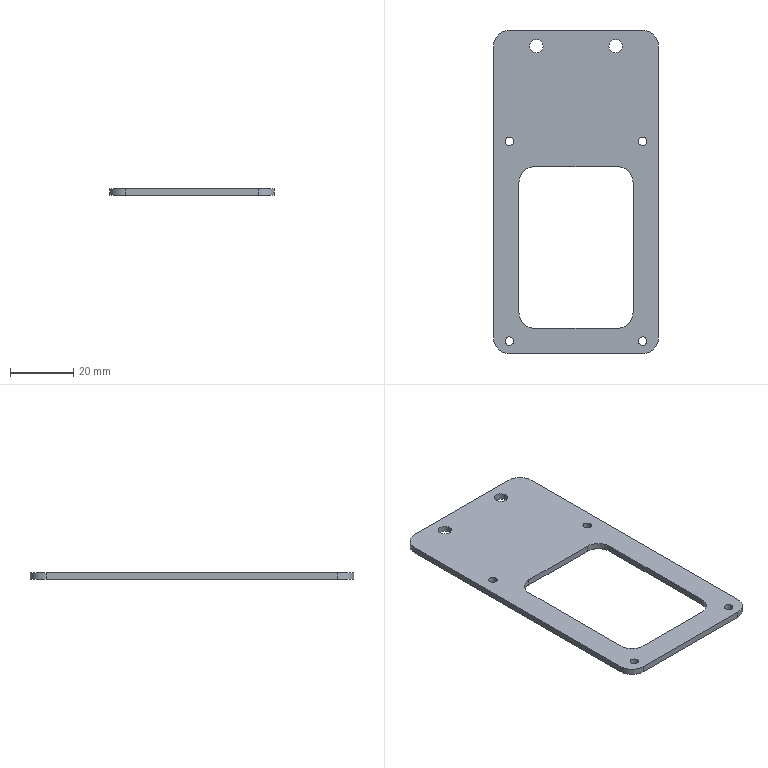Part | SolidWorks | features BaseBody 1 | 1 solid | 30 faces | box 52 x 102 x 2 mm | volume 6835 mm3 | cylinder 20 | plane 10 | commonest cylinder face diameters 2.7 x8 10 x8 4.2 x4
STEP:
#1=CARTESIAN_POINT('',(-14.6,46.,0.));
#2=VERTEX_POINT('',#1);
#3=CARTESIAN_POINT('',(-10.4,46.,0.));
#4=VERTEX_POINT('',#3);
#5=CARTESIAN_POINT('',(-12.5,46.,0.));
#6=DIRECTION('',(0.,0.,1.));
#7=DIRECTION('',(1.,0.,0.));
#8=AXIS2_PLACEMENT_3D('',#5,#6,#7);
#9=CIRCLE('',#8,2.1);
#10=EDGE_CURVE('',#2,#4,#9,.T.);
#11=ORIENTED_EDGE('',*,*,#10,.F.);
#12=CARTESIAN_POINT('',(-14.6,46.,2.));
#13=VERTEX_POINT('',#12);
#14=CARTESIAN_POINT('',(-14.6,46.,0.));
#15=DIRECTION('',(0.,0.,1.));
#16=VECTOR('',#15,1000.);
#17=LINE('',#14,#16);
#18=EDGE_CURVE('',#2,#13,#17,.T.);
#19=ORIENTED_EDGE('',*,*,#18,.T.);
#20=CARTESIAN_POINT('',(-10.4,46.,2.));
#21=VERTEX_POINT('',#20);
#22=CARTESIAN_POINT('',(-12.5,46.,2.));
#23=DIRECTION('',(0.,0.,1.));
#24=DIRECTION('',(1.,0.,0.));
#25=AXIS2_PLACEMENT_3D('',#22,#23,#24);
#26=CIRCLE('',#25,2.1);
#27=EDGE_CURVE('',#13,#21,#26,.T.);
#28=ORIENTED_EDGE('',*,*,#27,.T.);
#29=CARTESIAN_POINT('',(-10.4,46.,0.));
#30=DIRECTION('',(0.,0.,1.));
#31=VECTOR('',#30,1000.);
#32=LINE('',#29,#31);
#33=EDGE_CURVE('',#4,#21,#32,.T.);
#34=ORIENTED_EDGE('',*,*,#33,.F.);
#35=EDGE_LOOP('',(#11,#19,#28,#34));
#36=FACE_OUTER_BOUND('',#35,.T.);
#37=CARTESIAN_POINT('',(-12.5,46.,0.));
#38=DIRECTION('',(0.,0.,1.));
#39=DIRECTION('',(1.,0.,0.));
#40=AXIS2_PLACEMENT_3D('',#37,#38,#39);
#41=CYLINDRICAL_SURFACE('',#40,2.1);
#42=ADVANCED_FACE('',(#36),#41,.F.);
#43=CARTESIAN_POINT('',(19.65,-47.,0.));
#44=VERTEX_POINT('',#43);
#45=CARTESIAN_POINT('',(22.35,-47.,0.));
#46=VERTEX_POINT('',#45);
#47=CARTESIAN_POINT('',(21.,-47.,0.));
#48=DIRECTION('',(0.,0.,1.));
#49=DIRECTION('',(1.,0.,0.));
#50=AXIS2_PLACEMENT_3D('',#47,#48,#49);
#51=CIRCLE('',#50,1.35);
#52=EDGE_CURVE('',#44,#46,#51,.T.);
#53=ORIENTED_EDGE('',*,*,#52,.F.);
#54=CARTESIAN_POINT('',(19.65,-47.,2.));
#55=VERTEX_POINT('',#54);
#56=CARTESIAN_POINT('',(19.65,-47.,0.));
#57=DIRECTION('',(0.,0.,1.));
#58=VECTOR('',#57,1000.);
#59=LINE('',#56,#58);
#60=EDGE_CURVE('',#44,#55,#59,.T.);
#61=ORIENTED_EDGE('',*,*,#60,.T.);
#62=CARTESIAN_POINT('',(22.35,-47.,2.));
#63=VERTEX_POINT('',#62);
#64=CARTESIAN_POINT('',(21.,-47.,2.));
#65=DIRECTION('',(0.,0.,1.));
#66=DIRECTION('',(1.,0.,0.));
#67=AXIS2_PLACEMENT_3D('',#64,#65,#66);
#68=CIRCLE('',#67,1.35);
#69=EDGE_CURVE('',#55,#63,#68,.T.);
#70=ORIENTED_EDGE('',*,*,#69,.T.);
#71=CARTESIAN_POINT('',(22.35,-47.,0.));
#72=DIRECTION('',(0.,0.,1.));
#73=VECTOR('',#72,1000.);
#74=LINE('',#71,#73);
#75=EDGE_CURVE('',#46,#63,#74,.T.);
#76=ORIENTED_EDGE('',*,*,#75,.F.);
#77=EDGE_LOOP('',(#53,#61,#70,#76));
#78=FACE_OUTER_BOUND('',#77,.T.);
#79=CARTESIAN_POINT('',(21.,-47.,0.));
#80=DIRECTION('',(0.,0.,1.));
#81=DIRECTION('',(1.,0.,0.));
#82=AXIS2_PLACEMENT_3D('',#79,#80,#81);
#83=CYLINDRICAL_SURFACE('',#82,1.35);
#84=ADVANCED_FACE('',(#78),#83,.F.);
#85=CARTESIAN_POINT('',(10.4,46.,0.));
#86=VERTEX_POINT('',#85);
#87=CARTESIAN_POINT('',(14.6,46.,0.));
#88=VERTEX_POINT('',#87);
#89=CARTESIAN_POINT('',(12.5,46.,0.));
#90=DIRECTION('',(0.,0.,1.));
#91=DIRECTION('',(1.,0.,0.));
#92=AXIS2_PLACEMENT_3D('',#89,#90,#91);
#93=CIRCLE('',#92,2.1);
#94=EDGE_CURVE('',#86,#88,#93,.T.);
#95=ORIENTED_EDGE('',*,*,#94,.F.);
#96=CARTESIAN_POINT('',(10.4,46.,2.));
#97=VERTEX_POINT('',#96);
#98=CARTESIAN_POINT('',(10.4,46.,0.));
#99=DIRECTION('',(0.,0.,1.));
#100=VECTOR('',#99,1000.);
#101=LINE('',#98,#100);
#102=EDGE_CURVE('',#86,#97,#101,.T.);
#103=ORIENTED_EDGE('',*,*,#102,.T.);
#104=CARTESIAN_POINT('',(14.6,46.,2.));
#105=VERTEX_POINT('',#104);
#106=CARTESIAN_POINT('',(12.5,46.,2.));
#107=DIRECTION('',(0.,0.,1.));
#108=DIRECTION('',(1.,0.,0.));
#109=AXIS2_PLACEMENT_3D('',#106,#107,#108);
#110=CIRCLE('',#109,2.1);
#111=EDGE_CURVE('',#97,#105,#110,.T.);
#112=ORIENTED_EDGE('',*,*,#111,.T.);
#113=CARTESIAN_POINT('',(14.6,46.,0.));
#114=DIRECTION('',(0.,0.,1.));
#115=VECTOR('',#114,1000.);
#116=LINE('',#113,#115);
#117=EDGE_CURVE('',#88,#105,#116,.T.);
#118=ORIENTED_EDGE('',*,*,#117,.F.);
#119=EDGE_LOOP('',(#95,#103,#112,#118));
#120=FACE_OUTER_BOUND('',#119,.T.);
#121=CARTESIAN_POINT('',(12.5,46.,0.));
#122=DIRECTION('',(0.,0.,1.));
#123=DIRECTION('',(1.,0.,0.));
#124=AXIS2_PLACEMENT_3D('',#121,#122,#123);
#125=CYLINDRICAL_SURFACE('',#124,2.1);
#126=ADVANCED_FACE('',(#120),#125,.F.);
#127=CARTESIAN_POINT('',(-22.35,16.,0.));
#128=VERTEX_POINT('',#127);
#129=CARTESIAN_POINT('',(-19.65,16.,0.));
#130=VERTEX_POINT('',#129);
#131=CARTESIAN_POINT('',(-21.,16.,0.));
#132=DIRECTION('',(0.,0.,1.));
#133=DIRECTION('',(1.,0.,0.));
#134=AXIS2_PLACEMENT_3D('',#131,#132,#133);
#135=CIRCLE('',#134,1.35);
#136=EDGE_CURVE('',#128,#130,#135,.T.);
#137=ORIENTED_EDGE('',*,*,#136,.F.);
#138=CARTESIAN_POINT('',(-22.35,16.,2.));
#139=VERTEX_POINT('',#138);
#140=CARTESIAN_POINT('',(-22.35,16.,0.));
#141=DIRECTION('',(0.,0.,1.));
#142=VECTOR('',#141,1000.);
#143=LINE('',#140,#142);
#144=EDGE_CURVE('',#128,#139,#143,.T.);
#145=ORIENTED_EDGE('',*,*,#144,.T.);
#146=CARTESIAN_POINT('',(-19.65,16.,2.));
#147=VERTEX_POINT('',#146);
#148=CARTESIAN_POINT('',(-21.,16.,2.));
#149=DIRECTION('',(0.,0.,1.));
#150=DIRECTION('',(1.,0.,0.));
#151=AXIS2_PLACEMENT_3D('',#148,#149,#150);
#152=CIRCLE('',#151,1.35);
#153=EDGE_CURVE('',#139,#147,#152,.T.);
#154=ORIENTED_EDGE('',*,*,#153,.T.);
#155=CARTESIAN_POINT('',(-19.65,16.,0.));
#156=DIRECTION('',(0.,0.,1.));
#157=VECTOR('',#156,1000.);
#158=LINE('',#155,#157);
#159=EDGE_CURVE('',#130,#147,#158,.T.);
#160=ORIENTED_EDGE('',*,*,#159,.F.);
#161=EDGE_LOOP('',(#137,#145,#154,#160));
#162=FACE_OUTER_BOUND('',#161,.T.);
#163=CARTESIAN_POINT('',(-21.,16.,0.));
#164=DIRECTION('',(0.,0.,1.));
#165=DIRECTION('',(1.,0.,0.));
#166=AXIS2_PLACEMENT_3D('',#163,#164,#165);
#167=CYLINDRICAL_SURFACE('',#166,1.35);
#168=ADVANCED_FACE('',(#162),#167,.F.);
#169=CARTESIAN_POINT('',(19.65,16.,0.));
#170=VERTEX_POINT('',#169);
#171=CARTESIAN_POINT('',(22.35,16.,0.));
#172=VERTEX_POINT('',#171);
#173=CARTESIAN_POINT('',(21.,16.,0.));
#174=DIRECTION('',(0.,0.,1.));
#175=DIRECTION('',(1.,0.,0.));
#176=AXIS2_PLACEMENT_3D('',#173,#174,#175);
#177=CIRCLE('',#176,1.35);
#178=EDGE_CURVE('',#170,#172,#177,.T.);
#179=ORIENTED_EDGE('',*,*,#178,.F.);
#180=CARTESIAN_POINT('',(19.65,16.,2.));
#181=VERTEX_POINT('',#180);
#182=CARTESIAN_POINT('',(19.65,16.,0.));
#183=DIRECTION('',(0.,0.,1.));
#184=VECTOR('',#183,1000.);
#185=LINE('',#182,#184);
#186=EDGE_CURVE('',#170,#181,#185,.T.);
#187=ORIENTED_EDGE('',*,*,#186,.T.);
#188=CARTESIAN_POINT('',(22.35,16.,2.));
#189=VERTEX_POINT('',#188);
#190=CARTESIAN_POINT('',(21.,16.,2.));
#191=DIRECTION('',(0.,0.,1.));
#192=DIRECTION('',(1.,0.,0.));
#193=AXIS2_PLACEMENT_3D('',#190,#191,#192);
#194=CIRCLE('',#193,1.35);
#195=EDGE_CURVE('',#181,#189,#194,.T.);
#196=ORIENTED_EDGE('',*,*,#195,.T.);
#197=CARTESIAN_POINT('',(22.35,16.,0.));
#198=DIRECTION('',(0.,0.,1.));
#199=VECTOR('',#198,1000.);
#200=LINE('',#197,#199);
#201=EDGE_CURVE('',#172,#189,#200,.T.);
#202=ORIENTED_EDGE('',*,*,#201,.F.);
#203=EDGE_LOOP('',(#179,#187,#196,#202));
#204=FACE_OUTER_BOUND('',#203,.T.);
#205=CARTESIAN_POINT('',(21.,16.,0.));
#206=DIRECTION('',(0.,0.,1.));
#207=DIRECTION('',(1.,0.,0.));
#208=AXIS2_PLACEMENT_3D('',#205,#206,#207);
#209=CYLINDRICAL_SURFACE('',#208,1.35);
#210=ADVANCED_FACE('',(#204),#209,.F.);
#211=CARTESIAN_POINT('',(-22.35,-47.,0.));
#212=VERTEX_POINT('',#211);
#213=CARTESIAN_POINT('',(-19.65,-47.,0.));
#214=VERTEX_POINT('',#213);
#215=CARTESIAN_POINT('',(-21.,-47.,0.));
#216=DIRECTION('',(0.,0.,1.));
#217=DIRECTION('',(1.,0.,0.));
#218=AXIS2_PLACEMENT_3D('',#215,#216,#217);
#219=CIRCLE('',#218,1.35);
#220=EDGE_CURVE('',#212,#214,#219,.T.);
#221=ORIENTED_EDGE('',*,*,#220,.F.);
#222=CARTESIAN_POINT('',(-22.35,-47.,2.));
#223=VERTEX_POINT('',#222);
#224=CARTESIAN_POINT('',(-22.35,-47.,0.));
#225=DIRECTION('',(0.,0.,1.));
#226=VECTOR('',#225,1000.);
#227=LINE('',#224,#226);
#228=EDGE_CURVE('',#212,#223,#227,.T.);
#229=ORIENTED_EDGE('',*,*,#228,.T.);
#230=CARTESIAN_POINT('',(-19.65,-47.,2.));
#231=VERTEX_POINT('',#230);
#232=CARTESIAN_POINT('',(-21.,-47.,2.));
#233=DIRECTION('',(0.,0.,1.));
#234=DIRECTION('',(1.,0.,0.));
#235=AXIS2_PLACEMENT_3D('',#232,#233,#234);
#236=CIRCLE('',#235,1.35);
#237=EDGE_CURVE('',#223,#231,#236,.T.);
#238=ORIENTED_EDGE('',*,*,#237,.T.);
#239=CARTESIAN_POINT('',(-19.65,-47.,0.));
#240=DIRECTION('',(0.,0.,1.));
#241=VECTOR('',#240,1000.);
#242=LINE('',#239,#241);
#243=EDGE_CURVE('',#214,#231,#242,.T.);
#244=ORIENTED_EDGE('',*,*,#243,.F.);
#245=EDGE_LOOP('',(#221,#229,#238,#244));
#246=FACE_OUTER_BOUND('',#245,.T.);
#247=CARTESIAN_POINT('',(-21.,-47.,0.));
#248=DIRECTION('',(0.,0.,1.));
#249=DIRECTION('',(1.,0.,0.));
#250=AXIS2_PLACEMENT_3D('',#247,#248,#249);
#251=CYLINDRICAL_SURFACE('',#250,1.35);
#252=ADVANCED_FACE('',(#246),#251,.F.);
#253=CARTESIAN_POINT('',(-21.,-51.,2.));
#254=VERTEX_POINT('',#253);
#255=CARTESIAN_POINT('',(-26.,-46.,2.));
#256=VERTEX_POINT('',#255);
#257=CARTESIAN_POINT('',(-21.,-46.,2.));
#258=DIRECTION('',(0.,0.,-1.));
#259=DIRECTION('',(-1.,0.,0.));
#260=AXIS2_PLACEMENT_3D('',#257,#258,#259);
#261=CIRCLE('',#260,5.);
#262=EDGE_CURVE('',#254,#256,#261,.T.);
#263=ORIENTED_EDGE('',*,*,#262,.F.);
#264=CARTESIAN_POINT('',(21.,-51.,2.));
#265=VERTEX_POINT('',#264);
#266=CARTESIAN_POINT('',(0.,-51.,2.));
#267=DIRECTION('',(-1.,0.,0.));
#268=VECTOR('',#267,1000.);
#269=LINE('',#266,#268);
#270=EDGE_CURVE('',#265,#254,#269,.T.);
#271=ORIENTED_EDGE('',*,*,#270,.F.);
#272=CARTESIAN_POINT('',(26.,-46.,2.));
#273=VERTEX_POINT('',#272);
#274=CARTESIAN_POINT('',(21.,-46.,2.));
#275=DIRECTION('',(0.,0.,-1.));
#276=DIRECTION('',(-1.,0.,0.));
#277=AXIS2_PLACEMENT_3D('',#274,#275,#276);
#278=CIRCLE('',#277,5.);
#279=EDGE_CURVE('',#273,#265,#278,.T.);
#280=ORIENTED_EDGE('',*,*,#279,.F.);
#281=CARTESIAN_POINT('',(26.,46.,2.));
#282=VERTEX_POINT('',#281);
#283=CARTESIAN_POINT('',(26.,0.,2.));
#284=DIRECTION('',(0.,-1.,0.));
#285=VECTOR('',#284,1000.);
#286=LINE('',#283,#285);
#287=EDGE_CURVE('',#282,#273,#286,.T.);
#288=ORIENTED_EDGE('',*,*,#287,.F.);
#289=CARTESIAN_POINT('',(21.,51.,2.));
#290=VERTEX_POINT('',#289);
#291=CARTESIAN_POINT('',(21.,46.,2.));
#292=DIRECTION('',(0.,0.,-1.));
#293=DIRECTION('',(-1.,0.,0.));
#294=AXIS2_PLACEMENT_3D('',#291,#292,#293);
#295=CIRCLE('',#294,5.);
#296=EDGE_CURVE('',#290,#282,#295,.T.);
#297=ORIENTED_EDGE('',*,*,#296,.F.);
#298=CARTESIAN_POINT('',(-21.,51.,2.));
#299=VERTEX_POINT('',#298);
#300=CARTESIAN_POINT('',(0.,51.,2.));
#301=DIRECTION('',(1.,0.,0.));
#302=VECTOR('',#301,1000.);
#303=LINE('',#300,#302);
#304=EDGE_CURVE('',#299,#290,#303,.T.);
#305=ORIENTED_EDGE('',*,*,#304,.F.);
#306=CARTESIAN_POINT('',(-26.,46.,2.));
#307=VERTEX_POINT('',#306);
#308=CARTESIAN_POINT('',(-21.,46.,2.));
#309=DIRECTION('',(0.,0.,-1.));
#310=DIRECTION('',(-1.,0.,0.));
#311=AXIS2_PLACEMENT_3D('',#308,#309,#310);
#312=CIRCLE('',#311,5.);
#313=EDGE_CURVE('',#307,#299,#312,.T.);
#314=ORIENTED_EDGE('',*,*,#313,.F.);
#315=CARTESIAN_POINT('',(-26.,0.,2.));
#316=DIRECTION('',(0.,1.,0.));
#317=VECTOR('',#316,1000.);
#318=LINE('',#315,#317);
#319=EDGE_CURVE('',#256,#307,#318,.T.);
#320=ORIENTED_EDGE('',*,*,#319,.F.);
#321=EDGE_LOOP('',(#263,#271,#280,#288,#297,#305,#314,#320));
#322=FACE_OUTER_BOUND('',#321,.T.);
#323=CARTESIAN_POINT('',(-12.5,46.,2.));
#324=DIRECTION('',(0.,0.,1.));
#325=DIRECTION('',(1.,0.,0.));
#326=AXIS2_PLACEMENT_3D('',#323,#324,#325);
#327=CIRCLE('',#326,2.1);
#328=EDGE_CURVE('',#21,#13,#327,.T.);
#329=ORIENTED_EDGE('',*,*,#328,.F.);
#330=ORIENTED_EDGE('',*,*,#27,.F.);
#331=EDGE_LOOP('',(#329,#330));
#332=FACE_BOUND('',#331,.T.);
#333=CARTESIAN_POINT('',(21.,-47.,2.));
#334=DIRECTION('',(0.,0.,1.));
#335=DIRECTION('',(1.,0.,0.));
#336=AXIS2_PLACEMENT_3D('',#333,#334,#335);
#337=CIRCLE('',#336,1.35);
#338=EDGE_CURVE('',#63,#55,#337,.T.);
#339=ORIENTED_EDGE('',*,*,#338,.F.);
#340=ORIENTED_EDGE('',*,*,#69,.F.);
#341=EDGE_LOOP('',(#339,#340));
#342=FACE_BOUND('',#341,.T.);
#343=CARTESIAN_POINT('',(12.5,46.,2.));
#344=DIRECTION('',(0.,0.,1.));
#345=DIRECTION('',(1.,0.,0.));
#346=AXIS2_PLACEMENT_3D('',#343,#344,#345);
#347=CIRCLE('',#346,2.1);
#348=EDGE_CURVE('',#105,#97,#347,.T.);
#349=ORIENTED_EDGE('',*,*,#348,.F.);
#350=ORIENTED_EDGE('',*,*,#111,.F.);
#351=EDGE_LOOP('',(#349,#350));
#352=FACE_BOUND('',#351,.T.);
#353=CARTESIAN_POINT('',(-21.,16.,2.));
#354=DIRECTION('',(0.,0.,1.));
#355=DIRECTION('',(1.,0.,0.));
#356=AXIS2_PLACEMENT_3D('',#353,#354,#355);
#357=CIRCLE('',#356,1.35);
#358=EDGE_CURVE('',#147,#139,#357,.T.);
#359=ORIENTED_EDGE('',*,*,#358,.F.);
#360=ORIENTED_EDGE('',*,*,#153,.F.);
#361=EDGE_LOOP('',(#359,#360));
#362=FACE_BOUND('',#361,.T.);
#363=CARTESIAN_POINT('',(21.,16.,2.));
#364=DIRECTION('',(0.,0.,1.));
#365=DIRECTION('',(1.,0.,0.));
#366=AXIS2_PLACEMENT_3D('',#363,#364,#365);
#367=CIRCLE('',#366,1.35);
#368=EDGE_CURVE('',#189,#181,#367,.T.);
#369=ORIENTED_EDGE('',*,*,#368,.F.);
#370=ORIENTED_EDGE('',*,*,#195,.F.);
#371=EDGE_LOOP('',(#369,#370));
#372=FACE_BOUND('',#371,.T.);
#373=CARTESIAN_POINT('',(-21.,-47.,2.));
#374=DIRECTION('',(0.,0.,1.));
#375=DIRECTION('',(1.,0.,0.));
#376=AXIS2_PLACEMENT_3D('',#373,#374,#375);
#377=CIRCLE('',#376,1.35);
#378=EDGE_CURVE('',#231,#223,#377,.T.);
#379=ORIENTED_EDGE('',*,*,#378,.F.);
#380=ORIENTED_EDGE('',*,*,#237,.F.);
#381=EDGE_LOOP('',(#379,#380));
#382=FACE_BOUND('',#381,.T.);
#383=CARTESIAN_POINT('',(18.,3.,2.));
#384=VERTEX_POINT('',#383);
#385=CARTESIAN_POINT('',(13.,8.,2.));
#386=VERTEX_POINT('',#385);
#387=CARTESIAN_POINT('',(13.,3.,2.));
#388=DIRECTION('',(0.,0.,1.));
#389=DIRECTION('',(-1.,0.,0.));
#390=AXIS2_PLACEMENT_3D('',#387,#388,#389);
#391=CIRCLE('',#390,5.);
#392=EDGE_CURVE('',#384,#386,#391,.T.);
#393=ORIENTED_EDGE('',*,*,#392,.F.);
#394=CARTESIAN_POINT('',(18.,-38.,2.));
#395=VERTEX_POINT('',#394);
#396=CARTESIAN_POINT('',(18.,0.,2.));
#397=DIRECTION('',(0.,1.,0.));
#398=VECTOR('',#397,1000.);
#399=LINE('',#396,#398);
#400=EDGE_CURVE('',#395,#384,#399,.T.);
#401=ORIENTED_EDGE('',*,*,#400,.F.);
#402=CARTESIAN_POINT('',(13.,-43.,2.));
#403=VERTEX_POINT('',#402);
#404=CARTESIAN_POINT('',(13.,-38.,2.));
#405=DIRECTION('',(0.,0.,1.));
#406=DIRECTION('',(-1.,0.,0.));
#407=AXIS2_PLACEMENT_3D('',#404,#405,#406);
#408=CIRCLE('',#407,5.);
#409=EDGE_CURVE('',#403,#395,#408,.T.);
#410=ORIENTED_EDGE('',*,*,#409,.F.);
#411=CARTESIAN_POINT('',(-13.,-43.,2.));
#412=VERTEX_POINT('',#411);
#413=CARTESIAN_POINT('',(0.,-43.,2.));
#414=DIRECTION('',(1.,0.,0.));
#415=VECTOR('',#414,1000.);
#416=LINE('',#413,#415);
#417=EDGE_CURVE('',#412,#403,#416,.T.);
#418=ORIENTED_EDGE('',*,*,#417,.F.);
#419=CARTESIAN_POINT('',(-18.,-38.,2.));
#420=VERTEX_POINT('',#419);
#421=CARTESIAN_POINT('',(-13.,-38.,2.));
#422=DIRECTION('',(0.,0.,1.));
#423=DIRECTION('',(-1.,0.,0.));
#424=AXIS2_PLACEMENT_3D('',#421,#422,#423);
#425=CIRCLE('',#424,5.);
#426=EDGE_CURVE('',#420,#412,#425,.T.);
#427=ORIENTED_EDGE('',*,*,#426,.F.);
#428=CARTESIAN_POINT('',(-18.,3.,2.));
#429=VERTEX_POINT('',#428);
#430=CARTESIAN_POINT('',(-18.,0.,2.));
#431=DIRECTION('',(0.,-1.,0.));
#432=VECTOR('',#431,1000.);
#433=LINE('',#430,#432);
#434=EDGE_CURVE('',#429,#420,#433,.T.);
#435=ORIENTED_EDGE('',*,*,#434,.F.);
#436=CARTESIAN_POINT('',(-13.,8.,2.));
#437=VERTEX_POINT('',#436);
#438=CARTESIAN_POINT('',(-13.,3.,2.));
#439=DIRECTION('',(0.,0.,1.));
#440=DIRECTION('',(-1.,0.,0.));
#441=AXIS2_PLACEMENT_3D('',#438,#439,#440);
#442=CIRCLE('',#441,5.);
#443=EDGE_CURVE('',#437,#429,#442,.T.);
#444=ORIENTED_EDGE('',*,*,#443,.F.);
#445=CARTESIAN_POINT('',(0.,8.,2.));
#446=DIRECTION('',(-1.,0.,0.));
#447=VECTOR('',#446,1000.);
#448=LINE('',#445,#447);
#449=EDGE_CURVE('',#386,#437,#448,.T.);
#450=ORIENTED_EDGE('',*,*,#449,.F.);
#451=EDGE_LOOP('',(#393,#401,#410,#418,#427,#435,#444,#450));
#452=FACE_BOUND('',#451,.T.);
#453=CARTESIAN_POINT('',(0.,0.,2.));
#454=DIRECTION('',(0.,0.,-1.));
#455=DIRECTION('',(-1.,0.,0.));
#456=AXIS2_PLACEMENT_3D('',#453,#454,#455);
#457=PLANE('',#456);
#458=ADVANCED_FACE('',(#322,#332,#342,#352,#362,#372,#382,#452),#457,.F.);
#459=CARTESIAN_POINT('',(-26.,-46.,0.));
#460=VERTEX_POINT('',#459);
#461=CARTESIAN_POINT('',(-26.,-46.,2.));
#462=DIRECTION('',(0.,0.,-1.));
#463=VECTOR('',#462,1000.);
#464=LINE('',#461,#463);
#465=EDGE_CURVE('',#256,#460,#464,.T.);
#466=ORIENTED_EDGE('',*,*,#465,.F.);
#467=ORIENTED_EDGE('',*,*,#319,.T.);
#468=CARTESIAN_POINT('',(-26.,46.,0.));
#469=VERTEX_POINT('',#468);
#470=CARTESIAN_POINT('',(-26.,46.,2.));
#471=DIRECTION('',(0.,0.,1.));
#472=VECTOR('',#471,1000.);
#473=LINE('',#470,#472);
#474=EDGE_CURVE('',#469,#307,#473,.T.);
#475=ORIENTED_EDGE('',*,*,#474,.F.);
#476=CARTESIAN_POINT('',(-26.,-51.,0.));
#477=DIRECTION('',(0.,1.,0.));
#478=VECTOR('',#477,1000.);
#479=LINE('',#476,#478);
#480=EDGE_CURVE('',#460,#469,#479,.T.);
#481=ORIENTED_EDGE('',*,*,#480,.F.);
#482=EDGE_LOOP('',(#466,#467,#475,#481));
#483=FACE_OUTER_BOUND('',#482,.T.);
#484=CARTESIAN_POINT('',(-26.,-51.,2.));
#485=DIRECTION('',(1.,0.,0.));
#486=DIRECTION('',(0.,0.,-1.));
#487=AXIS2_PLACEMENT_3D('',#484,#485,#486);
#488=PLANE('',#487);
#489=ADVANCED_FACE('',(#483),#488,.F.);
#490=CARTESIAN_POINT('',(-21.,-51.,0.));
#491=VERTEX_POINT('',#490);
#492=CARTESIAN_POINT('',(-21.,-46.,0.));
#493=DIRECTION('',(0.,0.,1.));
#494=DIRECTION('',(-1.,0.,0.));
#495=AXIS2_PLACEMENT_3D('',#492,#493,#494);
#496=CIRCLE('',#495,5.);
#497=EDGE_CURVE('',#460,#491,#496,.T.);
#498=ORIENTED_EDGE('',*,*,#497,.T.);
#499=CARTESIAN_POINT('',(-21.,-51.,2.));
#500=DIRECTION('',(0.,0.,1.));
#501=VECTOR('',#500,1000.);
#502=LINE('',#499,#501);
#503=EDGE_CURVE('',#491,#254,#502,.T.);
#504=ORIENTED_EDGE('',*,*,#503,.T.);
#505=ORIENTED_EDGE('',*,*,#262,.T.);
#506=ORIENTED_EDGE('',*,*,#465,.T.);
#507=EDGE_LOOP('',(#498,#504,#505,#506));
#508=FACE_OUTER_BOUND('',#507,.T.);
#509=CARTESIAN_POINT('',(-21.,-46.,2.));
#510=DIRECTION('',(0.,0.,-1.));
#511=DIRECTION('',(-1.,0.,0.));
#512=AXIS2_PLACEMENT_3D('',#509,#510,#511);
#513=CYLINDRICAL_SURFACE('',#512,5.);
#514=ADVANCED_FACE('',(#508),#513,.T.);
#515=ORIENTED_EDGE('',*,*,#503,.F.);
#516=CARTESIAN_POINT('',(21.,-51.,0.));
#517=VERTEX_POINT('',#516);
#518=CARTESIAN_POINT('',(-26.,-51.,0.));
#519=DIRECTION('',(-1.,0.,0.));
#520=VECTOR('',#519,1000.);
#521=LINE('',#518,#520);
#522=EDGE_CURVE('',#517,#491,#521,.T.);
#523=ORIENTED_EDGE('',*,*,#522,.F.);
#524=CARTESIAN_POINT('',(21.,-51.,2.));
#525=DIRECTION('',(0.,0.,-1.));
#526=VECTOR('',#525,1000.);
#527=LINE('',#524,#526);
#528=EDGE_CURVE('',#265,#517,#527,.T.);
#529=ORIENTED_EDGE('',*,*,#528,.F.);
#530=ORIENTED_EDGE('',*,*,#270,.T.);
#531=EDGE_LOOP('',(#515,#523,#529,#530));
#532=FACE_OUTER_BOUND('',#531,.T.);
#533=CARTESIAN_POINT('',(-26.,-51.,2.));
#534=DIRECTION('',(0.,1.,0.));
#535=DIRECTION('',(0.,0.,1.));
#536=AXIS2_PLACEMENT_3D('',#533,#534,#535);
#537=PLANE('',#536);
#538=ADVANCED_FACE('',(#532),#537,.F.);
#539=CARTESIAN_POINT('',(26.,-46.,0.));
#540=VERTEX_POINT('',#539);
#541=CARTESIAN_POINT('',(21.,-46.,0.));
#542=DIRECTION('',(0.,0.,1.));
#543=DIRECTION('',(-1.,0.,0.));
#544=AXIS2_PLACEMENT_3D('',#541,#542,#543);
#545=CIRCLE('',#544,5.);
#546=EDGE_CURVE('',#517,#540,#545,.T.);
#547=ORIENTED_EDGE('',*,*,#546,.T.);
#548=CARTESIAN_POINT('',(26.,-46.,2.));
#549=DIRECTION('',(0.,0.,1.));
#550=VECTOR('',#549,1000.);
#551=LINE('',#548,#550);
#552=EDGE_CURVE('',#540,#273,#551,.T.);
#553=ORIENTED_EDGE('',*,*,#552,.T.);
#554=ORIENTED_EDGE('',*,*,#279,.T.);
#555=ORIENTED_EDGE('',*,*,#528,.T.);
#556=EDGE_LOOP('',(#547,#553,#554,#555));
#557=FACE_OUTER_BOUND('',#556,.T.);
#558=CARTESIAN_POINT('',(21.,-46.,2.));
#559=DIRECTION('',(0.,0.,-1.));
#560=DIRECTION('',(-1.,0.,0.));
#561=AXIS2_PLACEMENT_3D('',#558,#559,#560);
#562=CYLINDRICAL_SURFACE('',#561,5.);
#563=ADVANCED_FACE('',(#557),#562,.T.);
#564=ORIENTED_EDGE('',*,*,#552,.F.);
#565=CARTESIAN_POINT('',(26.,46.,0.));
#566=VERTEX_POINT('',#565);
#567=CARTESIAN_POINT('',(26.,-51.,0.));
#568=DIRECTION('',(0.,-1.,0.));
#569=VECTOR('',#568,1000.);
#570=LINE('',#567,#569);
#571=EDGE_CURVE('',#566,#540,#570,.T.);
#572=ORIENTED_EDGE('',*,*,#571,.F.);
#573=CARTESIAN_POINT('',(26.,46.,2.));
#574=DIRECTION('',(0.,0.,-1.));
#575=VECTOR('',#574,1000.);
#576=LINE('',#573,#575);
#577=EDGE_CURVE('',#282,#566,#576,.T.);
#578=ORIENTED_EDGE('',*,*,#577,.F.);
#579=ORIENTED_EDGE('',*,*,#287,.T.);
#580=EDGE_LOOP('',(#564,#572,#578,#579));
#581=FACE_OUTER_BOUND('',#580,.T.);
#582=CARTESIAN_POINT('',(26.,-51.,2.));
#583=DIRECTION('',(-1.,0.,0.));
#584=DIRECTION('',(0.,0.,1.));
#585=AXIS2_PLACEMENT_3D('',#582,#583,#584);
#586=PLANE('',#585);
#587=ADVANCED_FACE('',(#581),#586,.F.);
#588=CARTESIAN_POINT('',(21.,51.,0.));
#589=VERTEX_POINT('',#588);
#590=CARTESIAN_POINT('',(21.,46.,0.));
#591=DIRECTION('',(0.,0.,1.));
#592=DIRECTION('',(-1.,0.,0.));
#593=AXIS2_PLACEMENT_3D('',#590,#591,#592);
#594=CIRCLE('',#593,5.);
#595=EDGE_CURVE('',#566,#589,#594,.T.);
#596=ORIENTED_EDGE('',*,*,#595,.T.);
#597=CARTESIAN_POINT('',(21.,51.,2.));
#598=DIRECTION('',(0.,0.,1.));
#599=VECTOR('',#598,1000.);
#600=LINE('',#597,#599);
#601=EDGE_CURVE('',#589,#290,#600,.T.);
#602=ORIENTED_EDGE('',*,*,#601,.T.);
#603=ORIENTED_EDGE('',*,*,#296,.T.);
#604=ORIENTED_EDGE('',*,*,#577,.T.);
#605=EDGE_LOOP('',(#596,#602,#603,#604));
#606=FACE_OUTER_BOUND('',#605,.T.);
#607=CARTESIAN_POINT('',(21.,46.,2.));
#608=DIRECTION('',(0.,0.,-1.));
#609=DIRECTION('',(-1.,0.,0.));
#610=AXIS2_PLACEMENT_3D('',#607,#608,#609);
#611=CYLINDRICAL_SURFACE('',#610,5.);
#612=ADVANCED_FACE('',(#606),#611,.T.);
#613=CARTESIAN_POINT('',(-21.,51.,0.));
#614=VERTEX_POINT('',#613);
#615=CARTESIAN_POINT('',(-21.,51.,2.));
#616=DIRECTION('',(0.,0.,-1.));
#617=VECTOR('',#616,1000.);
#618=LINE('',#615,#617);
#619=EDGE_CURVE('',#299,#614,#618,.T.);
#620=ORIENTED_EDGE('',*,*,#619,.F.);
#621=ORIENTED_EDGE('',*,*,#304,.T.);
#622=ORIENTED_EDGE('',*,*,#601,.F.);
#623=CARTESIAN_POINT('',(-26.,51.,0.));
#624=DIRECTION('',(1.,0.,0.));
#625=VECTOR('',#624,1000.);
#626=LINE('',#623,#625);
#627=EDGE_CURVE('',#614,#589,#626,.T.);
#628=ORIENTED_EDGE('',*,*,#627,.F.);
#629=EDGE_LOOP('',(#620,#621,#622,#628));
#630=FACE_OUTER_BOUND('',#629,.T.);
#631=CARTESIAN_POINT('',(-26.,51.,2.));
#632=DIRECTION('',(0.,-1.,0.));
#633=DIRECTION('',(0.,0.,-1.));
#634=AXIS2_PLACEMENT_3D('',#631,#632,#633);
#635=PLANE('',#634);
#636=ADVANCED_FACE('',(#630),#635,.F.);
#637=CARTESIAN_POINT('',(-21.,46.,0.));
#638=DIRECTION('',(0.,0.,1.));
#639=DIRECTION('',(-1.,0.,0.));
#640=AXIS2_PLACEMENT_3D('',#637,#638,#639);
#641=CIRCLE('',#640,5.);
#642=EDGE_CURVE('',#614,#469,#641,.T.);
#643=ORIENTED_EDGE('',*,*,#642,.T.);
#644=ORIENTED_EDGE('',*,*,#474,.T.);
#645=ORIENTED_EDGE('',*,*,#313,.T.);
#646=ORIENTED_EDGE('',*,*,#619,.T.);
#647=EDGE_LOOP('',(#643,#644,#645,#646));
#648=FACE_OUTER_BOUND('',#647,.T.);
#649=CARTESIAN_POINT('',(-21.,46.,2.));
#650=DIRECTION('',(0.,0.,-1.));
#651=DIRECTION('',(-1.,0.,0.));
#652=AXIS2_PLACEMENT_3D('',#649,#650,#651);
#653=CYLINDRICAL_SURFACE('',#652,5.);
#654=ADVANCED_FACE('',(#648),#653,.T.);
#655=ORIENTED_EDGE('',*,*,#18,.F.);
#656=CARTESIAN_POINT('',(-12.5,46.,0.));
#657=DIRECTION('',(0.,0.,1.));
#658=DIRECTION('',(1.,0.,0.));
#659=AXIS2_PLACEMENT_3D('',#656,#657,#658);
#660=CIRCLE('',#659,2.1);
#661=EDGE_CURVE('',#4,#2,#660,.T.);
#662=ORIENTED_EDGE('',*,*,#661,.F.);
#663=ORIENTED_EDGE('',*,*,#33,.T.);
#664=ORIENTED_EDGE('',*,*,#328,.T.);
#665=EDGE_LOOP('',(#655,#662,#663,#664));
#666=FACE_OUTER_BOUND('',#665,.T.);
#667=CARTESIAN_POINT('',(-12.5,46.,0.));
#668=DIRECTION('',(0.,0.,1.));
#669=DIRECTION('',(1.,0.,0.));
#670=AXIS2_PLACEMENT_3D('',#667,#668,#669);
#671=CYLINDRICAL_SURFACE('',#670,2.1);
#672=ADVANCED_FACE('',(#666),#671,.F.);
#673=ORIENTED_EDGE('',*,*,#60,.F.);
#674=CARTESIAN_POINT('',(21.,-47.,0.));
#675=DIRECTION('',(0.,0.,1.));
#676=DIRECTION('',(1.,0.,0.));
#677=AXIS2_PLACEMENT_3D('',#674,#675,#676);
#678=CIRCLE('',#677,1.35);
#679=EDGE_CURVE('',#46,#44,#678,.T.);
#680=ORIENTED_EDGE('',*,*,#679,.F.);
#681=ORIENTED_EDGE('',*,*,#75,.T.);
#682=ORIENTED_EDGE('',*,*,#338,.T.);
#683=EDGE_LOOP('',(#673,#680,#681,#682));
#684=FACE_OUTER_BOUND('',#683,.T.);
#685=CARTESIAN_POINT('',(21.,-47.,0.));
#686=DIRECTION('',(0.,0.,1.));
#687=DIRECTION('',(1.,0.,0.));
#688=AXIS2_PLACEMENT_3D('',#685,#686,#687);
#689=CYLINDRICAL_SURFACE('',#688,1.35);
#690=ADVANCED_FACE('',(#684),#689,.F.);
#691=ORIENTED_EDGE('',*,*,#102,.F.);
#692=CARTESIAN_POINT('',(12.5,46.,0.));
#693=DIRECTION('',(0.,0.,1.));
#694=DIRECTION('',(1.,0.,0.));
#695=AXIS2_PLACEMENT_3D('',#692,#693,#694);
#696=CIRCLE('',#695,2.1);
#697=EDGE_CURVE('',#88,#86,#696,.T.);
#698=ORIENTED_EDGE('',*,*,#697,.F.);
#699=ORIENTED_EDGE('',*,*,#117,.T.);
#700=ORIENTED_EDGE('',*,*,#348,.T.);
#701=EDGE_LOOP('',(#691,#698,#699,#700));
#702=FACE_OUTER_BOUND('',#701,.T.);
#703=CARTESIAN_POINT('',(12.5,46.,0.));
#704=DIRECTION('',(0.,0.,1.));
#705=DIRECTION('',(1.,0.,0.));
#706=AXIS2_PLACEMENT_3D('',#703,#704,#705);
#707=CYLINDRICAL_SURFACE('',#706,2.1);
#708=ADVANCED_FACE('',(#702),#707,.F.);
#709=ORIENTED_EDGE('',*,*,#144,.F.);
#710=CARTESIAN_POINT('',(-21.,16.,0.));
#711=DIRECTION('',(0.,0.,1.));
#712=DIRECTION('',(1.,0.,0.));
#713=AXIS2_PLACEMENT_3D('',#710,#711,#712);
#714=CIRCLE('',#713,1.35);
#715=EDGE_CURVE('',#130,#128,#714,.T.);
#716=ORIENTED_EDGE('',*,*,#715,.F.);
#717=ORIENTED_EDGE('',*,*,#159,.T.);
#718=ORIENTED_EDGE('',*,*,#358,.T.);
#719=EDGE_LOOP('',(#709,#716,#717,#718));
#720=FACE_OUTER_BOUND('',#719,.T.);
#721=CARTESIAN_POINT('',(-21.,16.,0.));
#722=DIRECTION('',(0.,0.,1.));
#723=DIRECTION('',(1.,0.,0.));
#724=AXIS2_PLACEMENT_3D('',#721,#722,#723);
#725=CYLINDRICAL_SURFACE('',#724,1.35);
#726=ADVANCED_FACE('',(#720),#725,.F.);
#727=ORIENTED_EDGE('',*,*,#186,.F.);
#728=CARTESIAN_POINT('',(21.,16.,0.));
#729=DIRECTION('',(0.,0.,1.));
#730=DIRECTION('',(1.,0.,0.));
#731=AXIS2_PLACEMENT_3D('',#728,#729,#730);
#732=CIRCLE('',#731,1.35);
#733=EDGE_CURVE('',#172,#170,#732,.T.);
#734=ORIENTED_EDGE('',*,*,#733,.F.);
#735=ORIENTED_EDGE('',*,*,#201,.T.);
#736=ORIENTED_EDGE('',*,*,#368,.T.);
#737=EDGE_LOOP('',(#727,#734,#735,#736));
#738=FACE_OUTER_BOUND('',#737,.T.);
#739=CARTESIAN_POINT('',(21.,16.,0.));
#740=DIRECTION('',(0.,0.,1.));
#741=DIRECTION('',(1.,0.,0.));
#742=AXIS2_PLACEMENT_3D('',#739,#740,#741);
#743=CYLINDRICAL_SURFACE('',#742,1.35);
#744=ADVANCED_FACE('',(#738),#743,.F.);
#745=ORIENTED_EDGE('',*,*,#228,.F.);
#746=CARTESIAN_POINT('',(-21.,-47.,0.));
#747=DIRECTION('',(0.,0.,1.));
#748=DIRECTION('',(1.,0.,0.));
#749=AXIS2_PLACEMENT_3D('',#746,#747,#748);
#750=CIRCLE('',#749,1.35);
#751=EDGE_CURVE('',#214,#212,#750,.T.);
#752=ORIENTED_EDGE('',*,*,#751,.F.);
#753=ORIENTED_EDGE('',*,*,#243,.T.);
#754=ORIENTED_EDGE('',*,*,#378,.T.);
#755=EDGE_LOOP('',(#745,#752,#753,#754));
#756=FACE_OUTER_BOUND('',#755,.T.);
#757=CARTESIAN_POINT('',(-21.,-47.,0.));
#758=DIRECTION('',(0.,0.,1.));
#759=DIRECTION('',(1.,0.,0.));
#760=AXIS2_PLACEMENT_3D('',#757,#758,#759);
#761=CYLINDRICAL_SURFACE('',#760,1.35);
#762=ADVANCED_FACE('',(#756),#761,.F.);
#763=CARTESIAN_POINT('',(-13.,8.,0.));
#764=VERTEX_POINT('',#763);
#765=CARTESIAN_POINT('',(-13.,8.,-8.));
#766=DIRECTION('',(0.,0.,1.));
#767=VECTOR('',#766,1000.);
#768=LINE('',#765,#767);
#769=EDGE_CURVE('',#764,#437,#768,.T.);
#770=ORIENTED_EDGE('',*,*,#769,.F.);
#771=CARTESIAN_POINT('',(13.,8.,0.));
#772=VERTEX_POINT('',#771);
#773=CARTESIAN_POINT('',(-18.,8.,0.));
#774=DIRECTION('',(-1.,0.,0.));
#775=VECTOR('',#774,1000.);
#776=LINE('',#773,#775);
#777=EDGE_CURVE('',#772,#764,#776,.T.);
#778=ORIENTED_EDGE('',*,*,#777,.F.);
#779=CARTESIAN_POINT('',(13.,8.,-8.));
#780=DIRECTION('',(0.,0.,-1.));
#781=VECTOR('',#780,1000.);
#782=LINE('',#779,#781);
#783=EDGE_CURVE('',#386,#772,#782,.T.);
#784=ORIENTED_EDGE('',*,*,#783,.F.);
#785=ORIENTED_EDGE('',*,*,#449,.T.);
#786=EDGE_LOOP('',(#770,#778,#784,#785));
#787=FACE_OUTER_BOUND('',#786,.T.);
#788=CARTESIAN_POINT('',(-18.,8.,-8.));
#789=DIRECTION('',(0.,1.,0.));
#790=DIRECTION('',(0.,0.,1.));
#791=AXIS2_PLACEMENT_3D('',#788,#789,#790);
#792=PLANE('',#791);
#793=ADVANCED_FACE('',(#787),#792,.F.);
#794=CARTESIAN_POINT('',(18.,3.,0.));
#795=VERTEX_POINT('',#794);
#796=CARTESIAN_POINT('',(18.,3.,-8.));
#797=DIRECTION('',(0.,0.,-1.));
#798=VECTOR('',#797,1000.);
#799=LINE('',#796,#798);
#800=EDGE_CURVE('',#384,#795,#799,.T.);
#801=ORIENTED_EDGE('',*,*,#800,.F.);
#802=ORIENTED_EDGE('',*,*,#392,.T.);
#803=ORIENTED_EDGE('',*,*,#783,.T.);
#804=CARTESIAN_POINT('',(13.,3.,0.));
#805=DIRECTION('',(0.,0.,1.));
#806=DIRECTION('',(-1.,0.,0.));
#807=AXIS2_PLACEMENT_3D('',#804,#805,#806);
#808=CIRCLE('',#807,5.);
#809=EDGE_CURVE('',#795,#772,#808,.T.);
#810=ORIENTED_EDGE('',*,*,#809,.F.);
#811=EDGE_LOOP('',(#801,#802,#803,#810));
#812=FACE_OUTER_BOUND('',#811,.T.);
#813=CARTESIAN_POINT('',(13.,3.,-8.));
#814=DIRECTION('',(0.,0.,-1.));
#815=DIRECTION('',(-1.,0.,0.));
#816=AXIS2_PLACEMENT_3D('',#813,#814,#815);
#817=CYLINDRICAL_SURFACE('',#816,5.);
#818=ADVANCED_FACE('',(#812),#817,.F.);
#819=CARTESIAN_POINT('',(18.,-38.,0.));
#820=VERTEX_POINT('',#819);
#821=CARTESIAN_POINT('',(18.,-38.,-8.));
#822=DIRECTION('',(0.,0.,-1.));
#823=VECTOR('',#822,1000.);
#824=LINE('',#821,#823);
#825=EDGE_CURVE('',#395,#820,#824,.T.);
#826=ORIENTED_EDGE('',*,*,#825,.F.);
#827=ORIENTED_EDGE('',*,*,#400,.T.);
#828=ORIENTED_EDGE('',*,*,#800,.T.);
#829=CARTESIAN_POINT('',(18.,8.,0.));
#830=DIRECTION('',(0.,1.,0.));
#831=VECTOR('',#830,1000.);
#832=LINE('',#829,#831);
#833=EDGE_CURVE('',#820,#795,#832,.T.);
#834=ORIENTED_EDGE('',*,*,#833,.F.);
#835=EDGE_LOOP('',(#826,#827,#828,#834));
#836=FACE_OUTER_BOUND('',#835,.T.);
#837=CARTESIAN_POINT('',(18.,8.,-8.));
#838=DIRECTION('',(1.,0.,0.));
#839=DIRECTION('',(0.,1.,0.));
#840=AXIS2_PLACEMENT_3D('',#837,#838,#839);
#841=PLANE('',#840);
#842=ADVANCED_FACE('',(#836),#841,.F.);
#843=CARTESIAN_POINT('',(13.,-43.,0.));
#844=VERTEX_POINT('',#843);
#845=CARTESIAN_POINT('',(13.,-43.,-8.));
#846=DIRECTION('',(0.,0.,-1.));
#847=VECTOR('',#846,1000.);
#848=LINE('',#845,#847);
#849=EDGE_CURVE('',#403,#844,#848,.T.);
#850=ORIENTED_EDGE('',*,*,#849,.F.);
#851=ORIENTED_EDGE('',*,*,#409,.T.);
#852=ORIENTED_EDGE('',*,*,#825,.T.);
#853=CARTESIAN_POINT('',(13.,-38.,0.));
#854=DIRECTION('',(0.,0.,1.));
#855=DIRECTION('',(-1.,0.,0.));
#856=AXIS2_PLACEMENT_3D('',#853,#854,#855);
#857=CIRCLE('',#856,5.);
#858=EDGE_CURVE('',#844,#820,#857,.T.);
#859=ORIENTED_EDGE('',*,*,#858,.F.);
#860=EDGE_LOOP('',(#850,#851,#852,#859));
#861=FACE_OUTER_BOUND('',#860,.T.);
#862=CARTESIAN_POINT('',(13.,-38.,-8.));
#863=DIRECTION('',(0.,0.,-1.));
#864=DIRECTION('',(-1.,0.,0.));
#865=AXIS2_PLACEMENT_3D('',#862,#863,#864);
#866=CYLINDRICAL_SURFACE('',#865,5.);
#867=ADVANCED_FACE('',(#861),#866,.F.);
#868=ORIENTED_EDGE('',*,*,#849,.T.);
#869=CARTESIAN_POINT('',(-13.,-43.,0.));
#870=VERTEX_POINT('',#869);
#871=CARTESIAN_POINT('',(-18.,-43.,0.));
#872=DIRECTION('',(1.,0.,0.));
#873=VECTOR('',#872,1000.);
#874=LINE('',#871,#873);
#875=EDGE_CURVE('',#870,#844,#874,.T.);
#876=ORIENTED_EDGE('',*,*,#875,.F.);
#877=CARTESIAN_POINT('',(-13.,-43.,-8.));
#878=DIRECTION('',(0.,0.,-1.));
#879=VECTOR('',#878,1000.);
#880=LINE('',#877,#879);
#881=EDGE_CURVE('',#412,#870,#880,.T.);
#882=ORIENTED_EDGE('',*,*,#881,.F.);
#883=ORIENTED_EDGE('',*,*,#417,.T.);
#884=EDGE_LOOP('',(#868,#876,#882,#883));
#885=FACE_OUTER_BOUND('',#884,.T.);
#886=CARTESIAN_POINT('',(-18.,-43.,-8.));
#887=DIRECTION('',(0.,-1.,0.));
#888=DIRECTION('',(0.,0.,-1.));
#889=AXIS2_PLACEMENT_3D('',#886,#887,#888);
#890=PLANE('',#889);
#891=ADVANCED_FACE('',(#885),#890,.F.);
#892=CARTESIAN_POINT('',(-18.,-38.,0.));
#893=VERTEX_POINT('',#892);
#894=CARTESIAN_POINT('',(-18.,-38.,-8.));
#895=DIRECTION('',(0.,0.,-1.));
#896=VECTOR('',#895,1000.);
#897=LINE('',#894,#896);
#898=EDGE_CURVE('',#420,#893,#897,.T.);
#899=ORIENTED_EDGE('',*,*,#898,.F.);
#900=ORIENTED_EDGE('',*,*,#426,.T.);
#901=ORIENTED_EDGE('',*,*,#881,.T.);
#902=CARTESIAN_POINT('',(-13.,-38.,0.));
#903=DIRECTION('',(0.,0.,1.));
#904=DIRECTION('',(-1.,0.,0.));
#905=AXIS2_PLACEMENT_3D('',#902,#903,#904);
#906=CIRCLE('',#905,5.);
#907=EDGE_CURVE('',#893,#870,#906,.T.);
#908=ORIENTED_EDGE('',*,*,#907,.F.);
#909=EDGE_LOOP('',(#899,#900,#901,#908));
#910=FACE_OUTER_BOUND('',#909,.T.);
#911=CARTESIAN_POINT('',(-13.,-38.,-8.));
#912=DIRECTION('',(0.,0.,-1.));
#913=DIRECTION('',(-1.,0.,0.));
#914=AXIS2_PLACEMENT_3D('',#911,#912,#913);
#915=CYLINDRICAL_SURFACE('',#914,5.);
#916=ADVANCED_FACE('',(#910),#915,.F.);
#917=ORIENTED_EDGE('',*,*,#898,.T.);
#918=CARTESIAN_POINT('',(-18.,3.,0.));
#919=VERTEX_POINT('',#918);
#920=CARTESIAN_POINT('',(-18.,8.,0.));
#921=DIRECTION('',(0.,-1.,0.));
#922=VECTOR('',#921,1000.);
#923=LINE('',#920,#922);
#924=EDGE_CURVE('',#919,#893,#923,.T.);
#925=ORIENTED_EDGE('',*,*,#924,.F.);
#926=CARTESIAN_POINT('',(-18.,3.,-8.));
#927=DIRECTION('',(0.,0.,-1.));
#928=VECTOR('',#927,1000.);
#929=LINE('',#926,#928);
#930=EDGE_CURVE('',#429,#919,#929,.T.);
#931=ORIENTED_EDGE('',*,*,#930,.F.);
#932=ORIENTED_EDGE('',*,*,#434,.T.);
#933=EDGE_LOOP('',(#917,#925,#931,#932));
#934=FACE_OUTER_BOUND('',#933,.T.);
#935=CARTESIAN_POINT('',(-18.,8.,-8.));
#936=DIRECTION('',(-1.,0.,0.));
#937=DIRECTION('',(0.,0.,1.));
#938=AXIS2_PLACEMENT_3D('',#935,#936,#937);
#939=PLANE('',#938);
#940=ADVANCED_FACE('',(#934),#939,.F.);
#941=ORIENTED_EDGE('',*,*,#769,.T.);
#942=ORIENTED_EDGE('',*,*,#443,.T.);
#943=ORIENTED_EDGE('',*,*,#930,.T.);
#944=CARTESIAN_POINT('',(-13.,3.,0.));
#945=DIRECTION('',(0.,0.,1.));
#946=DIRECTION('',(-1.,0.,0.));
#947=AXIS2_PLACEMENT_3D('',#944,#945,#946);
#948=CIRCLE('',#947,5.);
#949=EDGE_CURVE('',#764,#919,#948,.T.);
#950=ORIENTED_EDGE('',*,*,#949,.F.);
#951=EDGE_LOOP('',(#941,#942,#943,#950));
#952=FACE_OUTER_BOUND('',#951,.T.);
#953=CARTESIAN_POINT('',(-13.,3.,-8.));
#954=DIRECTION('',(0.,0.,-1.));
#955=DIRECTION('',(-1.,0.,0.));
#956=AXIS2_PLACEMENT_3D('',#953,#954,#955);
#957=CYLINDRICAL_SURFACE('',#956,5.);
#958=ADVANCED_FACE('',(#952),#957,.F.);
#959=ORIENTED_EDGE('',*,*,#571,.T.);
#960=ORIENTED_EDGE('',*,*,#546,.F.);
#961=ORIENTED_EDGE('',*,*,#522,.T.);
#962=ORIENTED_EDGE('',*,*,#497,.F.);
#963=ORIENTED_EDGE('',*,*,#480,.T.);
#964=ORIENTED_EDGE('',*,*,#642,.F.);
#965=ORIENTED_EDGE('',*,*,#627,.T.);
#966=ORIENTED_EDGE('',*,*,#595,.F.);
#967=EDGE_LOOP('',(#959,#960,#961,#962,#963,#964,#965,#966));
#968=FACE_OUTER_BOUND('',#967,.T.);
#969=ORIENTED_EDGE('',*,*,#661,.T.);
#970=ORIENTED_EDGE('',*,*,#10,.T.);
#971=EDGE_LOOP('',(#969,#970));
#972=FACE_BOUND('',#971,.T.);
#973=ORIENTED_EDGE('',*,*,#679,.T.);
#974=ORIENTED_EDGE('',*,*,#52,.T.);
#975=EDGE_LOOP('',(#973,#974));
#976=FACE_BOUND('',#975,.T.);
#977=ORIENTED_EDGE('',*,*,#697,.T.);
#978=ORIENTED_EDGE('',*,*,#94,.T.);
#979=EDGE_LOOP('',(#977,#978));
#980=FACE_BOUND('',#979,.T.);
#981=ORIENTED_EDGE('',*,*,#715,.T.);
#982=ORIENTED_EDGE('',*,*,#136,.T.);
#983=EDGE_LOOP('',(#981,#982));
#984=FACE_BOUND('',#983,.T.);
#985=ORIENTED_EDGE('',*,*,#733,.T.);
#986=ORIENTED_EDGE('',*,*,#178,.T.);
#987=EDGE_LOOP('',(#985,#986));
#988=FACE_BOUND('',#987,.T.);
#989=ORIENTED_EDGE('',*,*,#751,.T.);
#990=ORIENTED_EDGE('',*,*,#220,.T.);
#991=EDGE_LOOP('',(#989,#990));
#992=FACE_BOUND('',#991,.T.);
#993=ORIENTED_EDGE('',*,*,#875,.T.);
#994=ORIENTED_EDGE('',*,*,#858,.T.);
#995=ORIENTED_EDGE('',*,*,#833,.T.);
#996=ORIENTED_EDGE('',*,*,#809,.T.);
#997=ORIENTED_EDGE('',*,*,#777,.T.);
#998=ORIENTED_EDGE('',*,*,#949,.T.);
#999=ORIENTED_EDGE('',*,*,#924,.T.);
#1000=ORIENTED_EDGE('',*,*,#907,.T.);
#1001=EDGE_LOOP('',(#993,#994,#995,#996,#997,#998,#999,#1000));
#1002=FACE_BOUND('',#1001,.T.);
#1003=CARTESIAN_POINT('',(0.,0.,0.));
#1004=DIRECTION('',(0.,0.,-1.));
#1005=DIRECTION('',(-1.,0.,0.));
#1006=AXIS2_PLACEMENT_3D('',#1003,#1004,#1005);
#1007=PLANE('',#1006);
#1008=ADVANCED_FACE('',(#968,#972,#976,#980,#984,#988,#992,#1002),#1007,.T.);
#1009=CLOSED_SHELL('',(#42,#84,#126,#168,#210,#252,#458,#489,#514,#538,#563,#587,#612,#636,#654,#672,#690,#708,#726,#744,#762,#793,#818,#842,#867,#891,#916,#940,#958,#1008));
#1010=MANIFOLD_SOLID_BREP('',#1009);
#1011=CARTESIAN_POINT('',(0.,0.,0.));
#1012=DIRECTION('',(0.,0.,1.));
#1013=DIRECTION('',(1.,0.,0.));
#1014=AXIS2_PLACEMENT_3D('',#1011,#1012,#1013);
#1015=(LENGTH_UNIT()NAMED_UNIT(*)SI_UNIT(.MILLI.,.METRE.));
#1016=UNCERTAINTY_MEASURE_WITH_UNIT(LENGTH_MEASURE(0.00001),#1015,'','');
#1017=(NAMED_UNIT(*)PLANE_ANGLE_UNIT()SI_UNIT($,.RADIAN.));
#1018=(NAMED_UNIT(*)SI_UNIT($,.STERADIAN.)SOLID_ANGLE_UNIT());
#1019=(GEOMETRIC_REPRESENTATION_CONTEXT(3)GLOBAL_UNCERTAINTY_ASSIGNED_CONTEXT((#1016))GLOBAL_UNIT_ASSIGNED_CONTEXT((#1015,#1017,#1018))REPRESENTATION_CONTEXT('',''));
#1020=ADVANCED_BREP_SHAPE_REPRESENTATION('',(#1010,#1014),#1019);